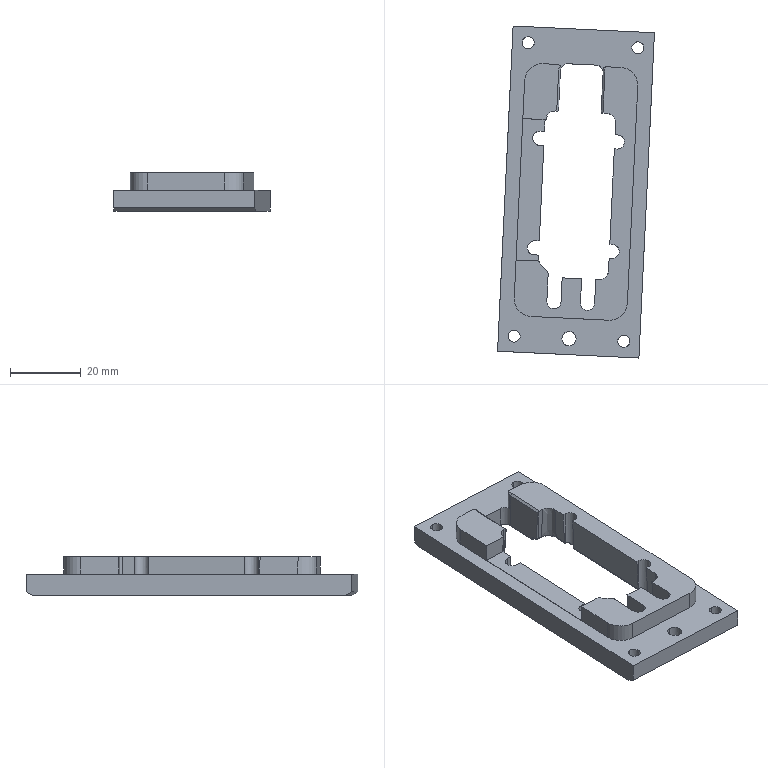Part | STEP file | X77-02601a | 1 solid | 279 faces | box 44.351 x 93.807 x 11.019 mm | volume 17666 mm3 | cylinder 119 | plane 83 | spline 69 | torus 3 | cone 3 | sphere 2 | commonest cylinder face diameters 1 x41 0.4 x26 4 x22 3.4 x8 6 x8 10 x5